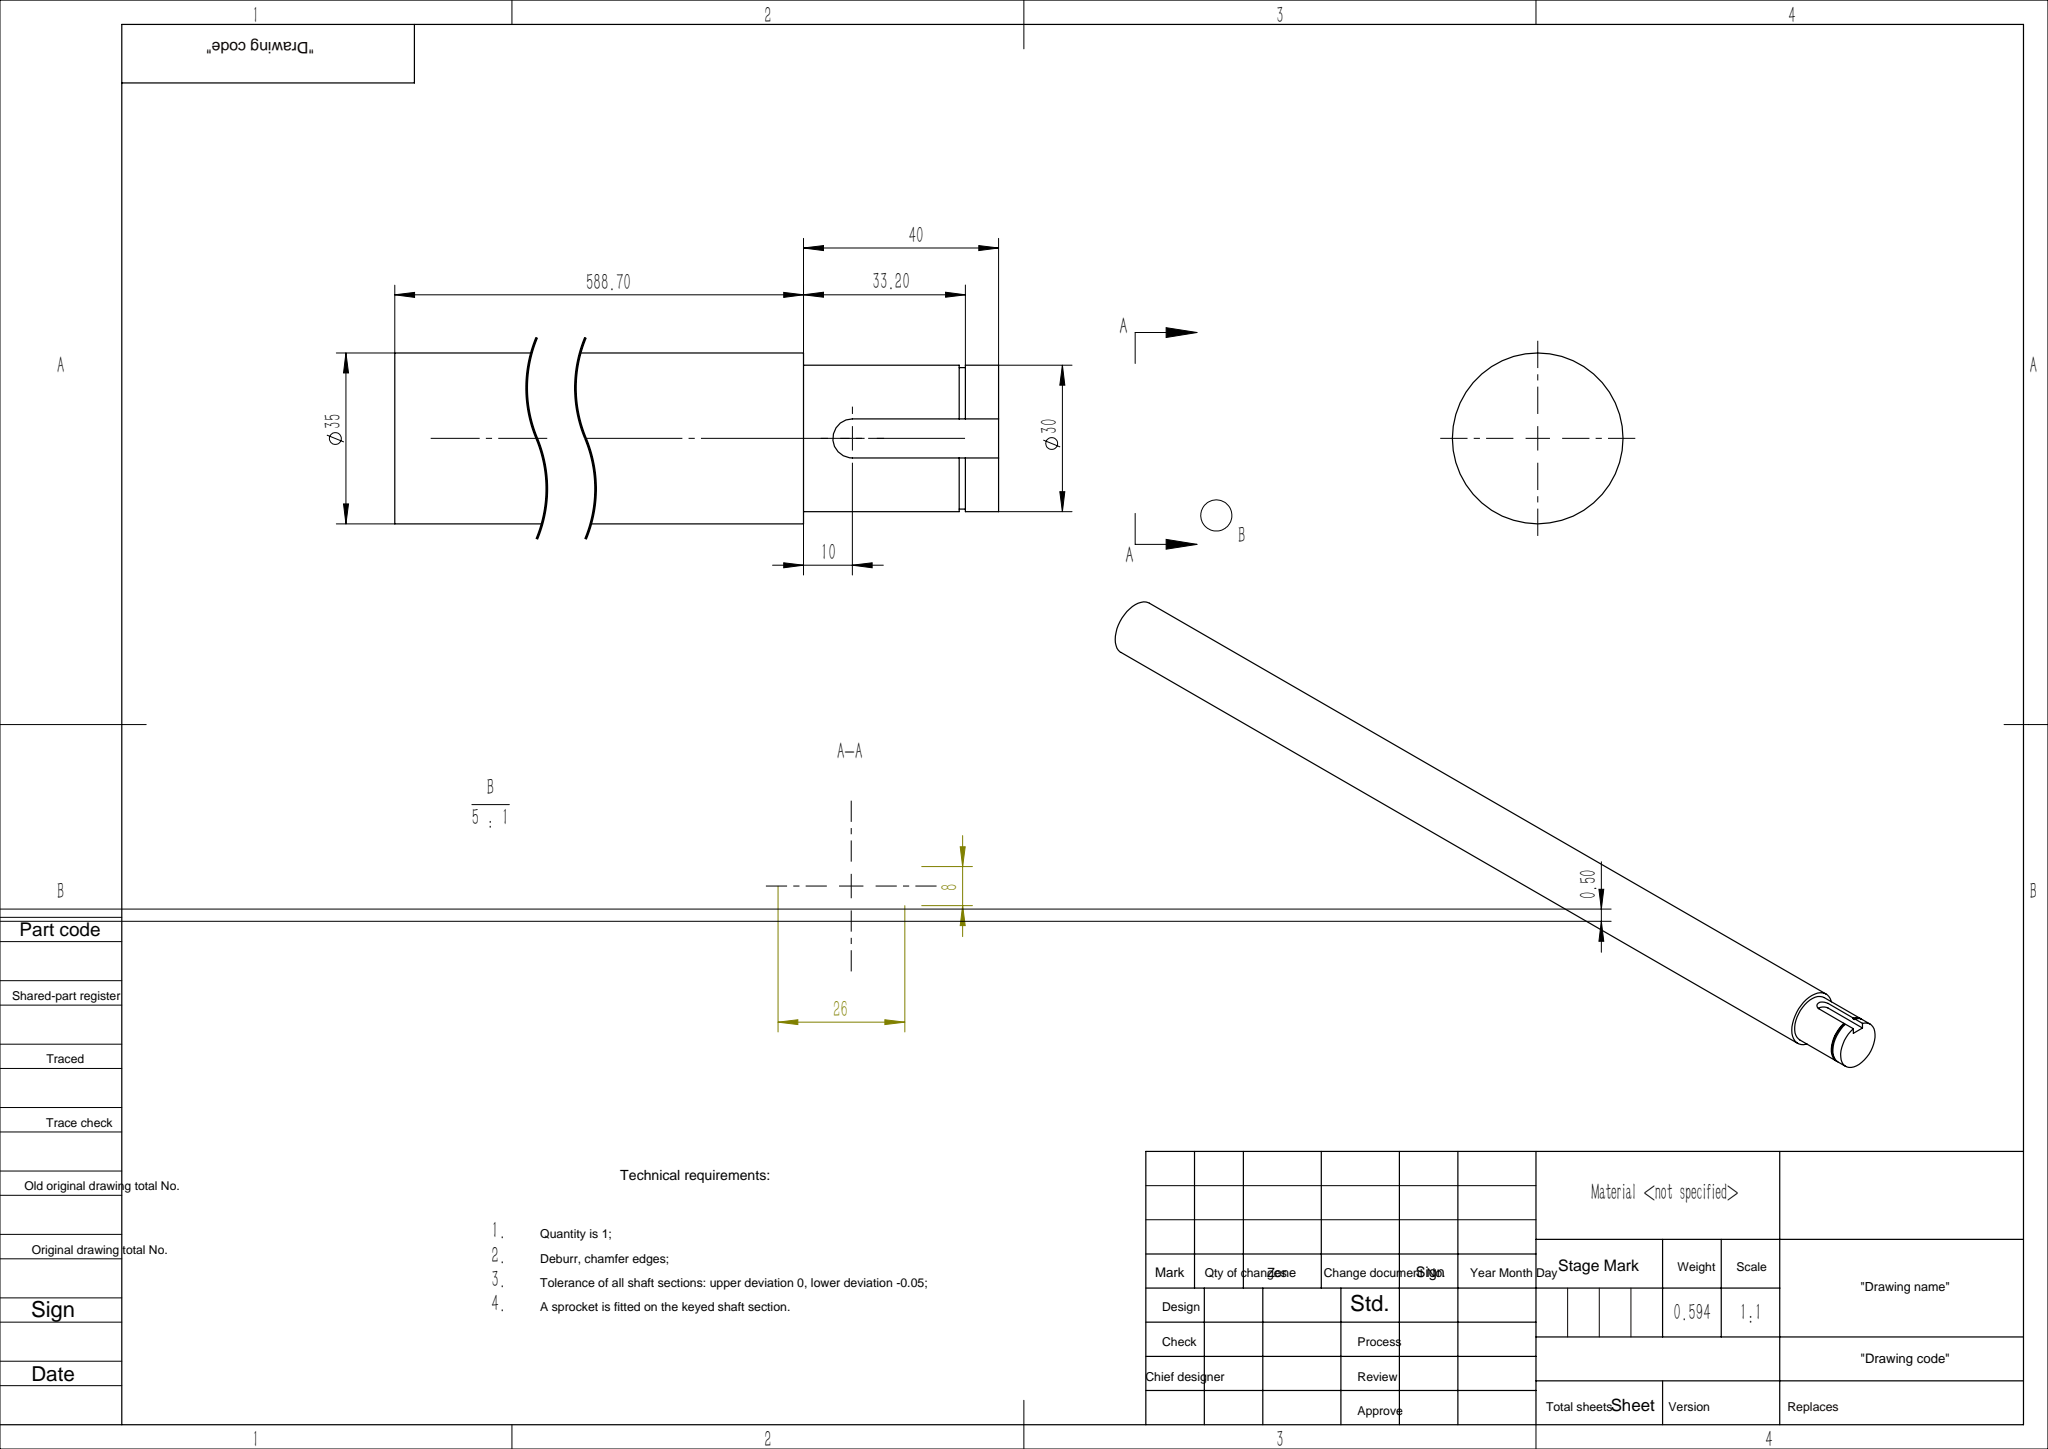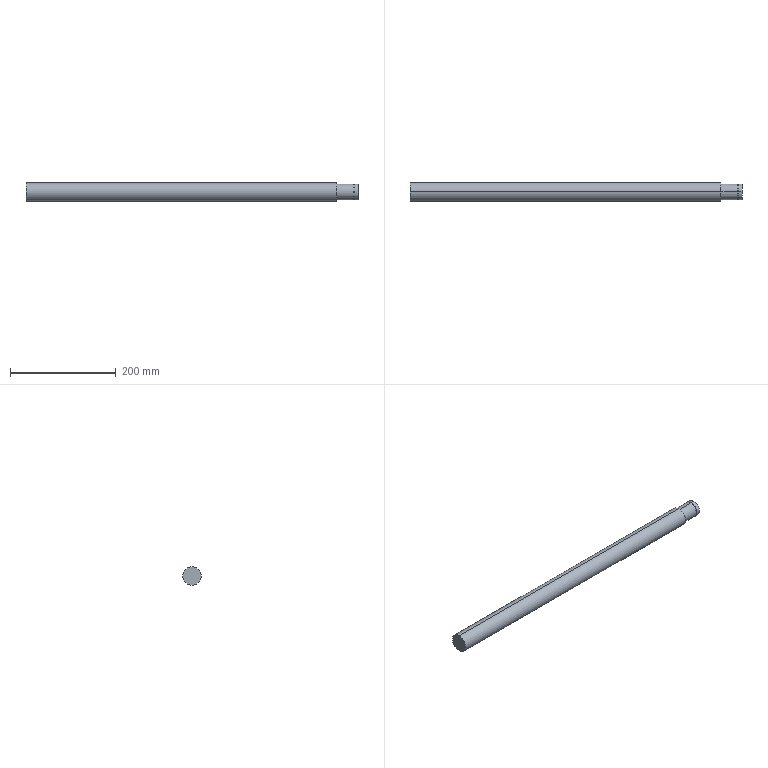Part | SolidWorks | features ICE 2, Cut 1, Extrusion 1 | 1 solid | 19 faces | box 628.7 x 35 x 35 mm | volume 593601 mm3 | cylinder 11 | plane 8 | commonest cylinder face diameters 30 x5 29 x3 35 x2 8 x1
STEP:
#1=CARTESIAN_POINT('',(620.6,13.937,4.));
#2=VERTEX_POINT('',#1);
#3=CARTESIAN_POINT('',(620.6,0.,14.5));
#4=VERTEX_POINT('',#3);
#5=CARTESIAN_POINT('',(620.6,0.,0.));
#6=DIRECTION('',(1.,0.,0.));
#7=DIRECTION('',(0.,0.,-1.));
#8=AXIS2_PLACEMENT_3D('',#5,#6,#7);
#9=CIRCLE('',#8,14.5);
#10=EDGE_CURVE('',#2,#4,#9,.T.);
#11=ORIENTED_EDGE('',*,*,#10,.T.);
#12=CARTESIAN_POINT('',(621.9,0.,14.5));
#13=VERTEX_POINT('',#12);
#14=CARTESIAN_POINT('',(620.6,0.,14.5));
#15=DIRECTION('',(1.,0.,0.));
#16=VECTOR('',#15,1000.);
#17=LINE('',#14,#16);
#18=EDGE_CURVE('',#4,#13,#17,.T.);
#19=ORIENTED_EDGE('',*,*,#18,.T.);
#20=CARTESIAN_POINT('',(621.9,13.937,4.));
#21=VERTEX_POINT('',#20);
#22=CARTESIAN_POINT('',(621.9,0.,0.));
#23=DIRECTION('',(1.,0.,0.));
#24=DIRECTION('',(0.,0.,-1.));
#25=AXIS2_PLACEMENT_3D('',#22,#23,#24);
#26=CIRCLE('',#25,14.5);
#27=EDGE_CURVE('',#21,#13,#26,.T.);
#28=ORIENTED_EDGE('',*,*,#27,.F.);
#29=CARTESIAN_POINT('',(620.6,13.937,4.));
#30=DIRECTION('',(-1.,0.,0.));
#31=VECTOR('',#30,1000.);
#32=LINE('',#29,#31);
#33=EDGE_CURVE('',#21,#2,#32,.T.);
#34=ORIENTED_EDGE('',*,*,#33,.T.);
#35=EDGE_LOOP('',(#11,#19,#28,#34));
#36=FACE_OUTER_BOUND('',#35,.T.);
#37=CARTESIAN_POINT('',(620.6,0.,0.));
#38=DIRECTION('',(1.,0.,0.));
#39=DIRECTION('',(0.,0.,-1.));
#40=AXIS2_PLACEMENT_3D('',#37,#38,#39);
#41=CYLINDRICAL_SURFACE('',#40,14.5);
#42=ADVANCED_FACE('',(#36),#41,.T.);
#43=ORIENTED_EDGE('',*,*,#18,.F.);
#44=CARTESIAN_POINT('',(620.6,0.,-14.5));
#45=VERTEX_POINT('',#44);
#46=CARTESIAN_POINT('',(620.6,0.,0.));
#47=DIRECTION('',(1.,0.,0.));
#48=DIRECTION('',(0.,0.,-1.));
#49=AXIS2_PLACEMENT_3D('',#46,#47,#48);
#50=CIRCLE('',#49,14.5);
#51=EDGE_CURVE('',#4,#45,#50,.T.);
#52=ORIENTED_EDGE('',*,*,#51,.T.);
#53=CARTESIAN_POINT('',(621.9,0.,-14.5));
#54=VERTEX_POINT('',#53);
#55=CARTESIAN_POINT('',(620.6,0.,-14.5));
#56=DIRECTION('',(1.,0.,0.));
#57=VECTOR('',#56,1000.);
#58=LINE('',#55,#57);
#59=EDGE_CURVE('',#45,#54,#58,.T.);
#60=ORIENTED_EDGE('',*,*,#59,.T.);
#61=CARTESIAN_POINT('',(621.9,0.,0.));
#62=DIRECTION('',(1.,0.,0.));
#63=DIRECTION('',(0.,0.,-1.));
#64=AXIS2_PLACEMENT_3D('',#61,#62,#63);
#65=CIRCLE('',#64,14.5);
#66=EDGE_CURVE('',#13,#54,#65,.T.);
#67=ORIENTED_EDGE('',*,*,#66,.F.);
#68=EDGE_LOOP('',(#43,#52,#60,#67));
#69=FACE_OUTER_BOUND('',#68,.T.);
#70=CARTESIAN_POINT('',(620.6,0.,0.));
#71=DIRECTION('',(1.,0.,0.));
#72=DIRECTION('',(0.,0.,-1.));
#73=AXIS2_PLACEMENT_3D('',#70,#71,#72);
#74=CYLINDRICAL_SURFACE('',#73,14.5);
#75=ADVANCED_FACE('',(#69),#74,.T.);
#76=CARTESIAN_POINT('',(621.9,14.457,4.));
#77=VERTEX_POINT('',#76);
#78=CARTESIAN_POINT('',(621.9,0.,15.));
#79=VERTEX_POINT('',#78);
#80=CARTESIAN_POINT('',(621.9,0.,0.));
#81=DIRECTION('',(1.,0.,0.));
#82=DIRECTION('',(0.,0.,-1.));
#83=AXIS2_PLACEMENT_3D('',#80,#81,#82);
#84=CIRCLE('',#83,15.);
#85=EDGE_CURVE('',#77,#79,#84,.T.);
#86=ORIENTED_EDGE('',*,*,#85,.T.);
#87=CARTESIAN_POINT('',(628.7,0.,15.));
#88=VERTEX_POINT('',#87);
#89=CARTESIAN_POINT('',(588.7,0.,15.));
#90=DIRECTION('',(1.,0.,0.));
#91=VECTOR('',#90,1000.);
#92=LINE('',#89,#91);
#93=EDGE_CURVE('',#79,#88,#92,.T.);
#94=ORIENTED_EDGE('',*,*,#93,.T.);
#95=CARTESIAN_POINT('',(628.7,14.457,4.));
#96=VERTEX_POINT('',#95);
#97=CARTESIAN_POINT('',(628.7,0.,0.));
#98=DIRECTION('',(1.,0.,0.));
#99=DIRECTION('',(0.,0.,-1.));
#100=AXIS2_PLACEMENT_3D('',#97,#98,#99);
#101=CIRCLE('',#100,15.);
#102=EDGE_CURVE('',#96,#88,#101,.T.);
#103=ORIENTED_EDGE('',*,*,#102,.F.);
#104=CARTESIAN_POINT('',(588.7,14.457,4.));
#105=DIRECTION('',(1.,0.,0.));
#106=VECTOR('',#105,1000.);
#107=LINE('',#104,#106);
#108=EDGE_CURVE('',#77,#96,#107,.T.);
#109=ORIENTED_EDGE('',*,*,#108,.F.);
#110=EDGE_LOOP('',(#86,#94,#103,#109));
#111=FACE_OUTER_BOUND('',#110,.T.);
#112=CARTESIAN_POINT('',(588.7,0.,0.));
#113=DIRECTION('',(1.,0.,0.));
#114=DIRECTION('',(0.,0.,-1.));
#115=AXIS2_PLACEMENT_3D('',#112,#113,#114);
#116=CYLINDRICAL_SURFACE('',#115,15.);
#117=ADVANCED_FACE('',(#111),#116,.T.);
#118=ORIENTED_EDGE('',*,*,#93,.F.);
#119=CARTESIAN_POINT('',(621.9,0.,-15.));
#120=VERTEX_POINT('',#119);
#121=CARTESIAN_POINT('',(621.9,0.,0.));
#122=DIRECTION('',(1.,0.,0.));
#123=DIRECTION('',(0.,0.,-1.));
#124=AXIS2_PLACEMENT_3D('',#121,#122,#123);
#125=CIRCLE('',#124,15.);
#126=EDGE_CURVE('',#79,#120,#125,.T.);
#127=ORIENTED_EDGE('',*,*,#126,.T.);
#128=CARTESIAN_POINT('',(628.7,0.,-15.));
#129=VERTEX_POINT('',#128);
#130=CARTESIAN_POINT('',(588.7,0.,-15.));
#131=DIRECTION('',(1.,0.,0.));
#132=VECTOR('',#131,1000.);
#133=LINE('',#130,#132);
#134=EDGE_CURVE('',#120,#129,#133,.T.);
#135=ORIENTED_EDGE('',*,*,#134,.T.);
#136=CARTESIAN_POINT('',(628.7,0.,0.));
#137=DIRECTION('',(1.,0.,0.));
#138=DIRECTION('',(0.,0.,-1.));
#139=AXIS2_PLACEMENT_3D('',#136,#137,#138);
#140=CIRCLE('',#139,15.);
#141=EDGE_CURVE('',#88,#129,#140,.T.);
#142=ORIENTED_EDGE('',*,*,#141,.F.);
#143=EDGE_LOOP('',(#118,#127,#135,#142));
#144=FACE_OUTER_BOUND('',#143,.T.);
#145=CARTESIAN_POINT('',(588.7,0.,0.));
#146=DIRECTION('',(1.,0.,0.));
#147=DIRECTION('',(0.,0.,-1.));
#148=AXIS2_PLACEMENT_3D('',#145,#146,#147);
#149=CYLINDRICAL_SURFACE('',#148,15.);
#150=ADVANCED_FACE('',(#144),#149,.T.);
#151=CARTESIAN_POINT('',(588.7,0.,-17.5));
#152=VERTEX_POINT('',#151);
#153=CARTESIAN_POINT('',(588.7,0.,17.5));
#154=VERTEX_POINT('',#153);
#155=CARTESIAN_POINT('',(588.7,0.,0.));
#156=DIRECTION('',(1.,0.,0.));
#157=DIRECTION('',(0.,0.,-1.));
#158=AXIS2_PLACEMENT_3D('',#155,#156,#157);
#159=CIRCLE('',#158,17.5);
#160=EDGE_CURVE('',#152,#154,#159,.T.);
#161=ORIENTED_EDGE('',*,*,#160,.F.);
#162=CARTESIAN_POINT('',(0.,0.,-17.5));
#163=VERTEX_POINT('',#162);
#164=CARTESIAN_POINT('',(628.7,0.,-17.5));
#165=DIRECTION('',(-1.,0.,0.));
#166=VECTOR('',#165,1000.);
#167=LINE('',#164,#166);
#168=EDGE_CURVE('',#152,#163,#167,.T.);
#169=ORIENTED_EDGE('',*,*,#168,.T.);
#170=CARTESIAN_POINT('',(0.,0.,17.5));
#171=VERTEX_POINT('',#170);
#172=CARTESIAN_POINT('',(0.,0.,0.));
#173=DIRECTION('',(1.,0.,0.));
#174=DIRECTION('',(0.,0.,-1.));
#175=AXIS2_PLACEMENT_3D('',#172,#173,#174);
#176=CIRCLE('',#175,17.5);
#177=EDGE_CURVE('',#163,#171,#176,.T.);
#178=ORIENTED_EDGE('',*,*,#177,.T.);
#179=CARTESIAN_POINT('',(628.7,0.,17.5));
#180=DIRECTION('',(-1.,0.,0.));
#181=VECTOR('',#180,1000.);
#182=LINE('',#179,#181);
#183=EDGE_CURVE('',#154,#171,#182,.T.);
#184=ORIENTED_EDGE('',*,*,#183,.F.);
#185=EDGE_LOOP('',(#161,#169,#178,#184));
#186=FACE_OUTER_BOUND('',#185,.T.);
#187=CARTESIAN_POINT('',(628.7,0.,0.));
#188=DIRECTION('',(-1.,0.,0.));
#189=DIRECTION('',(0.,0.,1.));
#190=AXIS2_PLACEMENT_3D('',#187,#188,#189);
#191=CYLINDRICAL_SURFACE('',#190,17.5);
#192=ADVANCED_FACE('',(#186),#191,.T.);
#193=CARTESIAN_POINT('',(588.7,0.,-15.));
#194=VERTEX_POINT('',#193);
#195=CARTESIAN_POINT('',(588.7,0.,15.));
#196=VERTEX_POINT('',#195);
#197=CARTESIAN_POINT('',(588.7,0.,0.));
#198=DIRECTION('',(1.,0.,0.));
#199=DIRECTION('',(0.,0.,-1.));
#200=AXIS2_PLACEMENT_3D('',#197,#198,#199);
#201=CIRCLE('',#200,15.);
#202=EDGE_CURVE('',#194,#196,#201,.T.);
#203=ORIENTED_EDGE('',*,*,#202,.T.);
#204=CARTESIAN_POINT('',(620.6,0.,15.));
#205=VERTEX_POINT('',#204);
#206=CARTESIAN_POINT('',(588.7,0.,15.));
#207=DIRECTION('',(1.,0.,0.));
#208=VECTOR('',#207,1000.);
#209=LINE('',#206,#208);
#210=EDGE_CURVE('',#196,#205,#209,.T.);
#211=ORIENTED_EDGE('',*,*,#210,.T.);
#212=CARTESIAN_POINT('',(620.6,14.457,4.));
#213=VERTEX_POINT('',#212);
#214=CARTESIAN_POINT('',(620.6,0.,0.));
#215=DIRECTION('',(1.,0.,0.));
#216=DIRECTION('',(0.,0.,-1.));
#217=AXIS2_PLACEMENT_3D('',#214,#215,#216);
#218=CIRCLE('',#217,15.);
#219=EDGE_CURVE('',#213,#205,#218,.T.);
#220=ORIENTED_EDGE('',*,*,#219,.F.);
#221=CARTESIAN_POINT('',(598.7,14.457,4.));
#222=VERTEX_POINT('',#221);
#223=CARTESIAN_POINT('',(588.7,14.457,4.));
#224=DIRECTION('',(1.,0.,0.));
#225=VECTOR('',#224,1000.);
#226=LINE('',#223,#225);
#227=EDGE_CURVE('',#222,#213,#226,.T.);
#228=ORIENTED_EDGE('',*,*,#227,.F.);
#229=CARTESIAN_POINT('',(598.7,14.457,-4.));
#230=VERTEX_POINT('',#229);
#231=CARTESIAN_POINT('',(598.7,14.457,-4.));
#232=CARTESIAN_POINT('',(598.434,14.457,-4.));
#233=CARTESIAN_POINT('',(598.174,14.464,-3.974));
#234=CARTESIAN_POINT('',(597.661,14.492,-3.872));
#235=CARTESIAN_POINT('',(597.406,14.513,-3.794));
#236=CARTESIAN_POINT('',(596.923,14.564,-3.593));
#237=CARTESIAN_POINT('',(596.693,14.594,-3.47));
#238=CARTESIAN_POINT('',(596.26,14.66,-3.18));
#239=CARTESIAN_POINT('',(596.055,14.696,-3.012));
#240=CARTESIAN_POINT('',(595.688,14.766,-2.645));
#241=CARTESIAN_POINT('',(595.523,14.801,-2.444));
#242=CARTESIAN_POINT('',(595.23,14.867,-2.008));
#243=CARTESIAN_POINT('',(595.107,14.896,-1.777));
#244=CARTESIAN_POINT('',(594.907,14.946,-1.296));
#245=CARTESIAN_POINT('',(594.829,14.966,-1.043));
#246=CARTESIAN_POINT('',(594.726,14.993,-0.5261));
#247=CARTESIAN_POINT('',(594.7,15.,-0.2658));
#248=CARTESIAN_POINT('',(594.7,15.,0.2585));
#249=CARTESIAN_POINT('',(594.726,14.993,0.5249));
#250=CARTESIAN_POINT('',(594.828,14.966,1.039));
#251=CARTESIAN_POINT('',(594.904,14.947,1.289));
#252=CARTESIAN_POINT('',(595.206,14.872,2.017));
#253=CARTESIAN_POINT('',(595.501,14.802,2.457));
#254=CARTESIAN_POINT('',(596.055,14.696,3.012));
#255=CARTESIAN_POINT('',(596.256,14.66,3.177));
#256=CARTESIAN_POINT('',(596.688,14.595,3.467));
#257=CARTESIAN_POINT('',(596.922,14.564,3.593));
#258=CARTESIAN_POINT('',(597.404,14.513,3.793));
#259=CARTESIAN_POINT('',(597.654,14.492,3.87));
#260=CARTESIAN_POINT('',(598.169,14.464,3.973));
#261=CARTESIAN_POINT('',(598.434,14.457,4.));
#262=CARTESIAN_POINT('',(598.7,14.457,4.));
#263=B_SPLINE_CURVE_WITH_KNOTS('',3,(#231,#232,#233,#234,#235,#236,#237,#238,#239,#240,#241,#242,#243,#244,#245,#246,#247,#248,#249,#250,#251,#252,#253,#254,#255,#256,#257,#258,#259,#260,#261,#262),.UNSPECIFIED.,.F.,.F.,(4,2,2,2,2,2,2,2,2,2,2,2,2,2,2,4),(0.,0.0007849,0.00157,0.002355,0.00314,0.003925,0.00471,0.005494,0.006279,0.007064,0.007849,0.009419,0.0102,0.01099,0.01177,0.01256),.UNSPECIFIED.);
#264=EDGE_CURVE('',#230,#222,#263,.T.);
#265=ORIENTED_EDGE('',*,*,#264,.F.);
#266=CARTESIAN_POINT('',(620.6,14.457,-4.));
#267=VERTEX_POINT('',#266);
#268=CARTESIAN_POINT('',(588.7,14.457,-4.));
#269=DIRECTION('',(-1.,0.,0.));
#270=VECTOR('',#269,1000.);
#271=LINE('',#268,#270);
#272=EDGE_CURVE('',#267,#230,#271,.T.);
#273=ORIENTED_EDGE('',*,*,#272,.F.);
#274=CARTESIAN_POINT('',(620.6,0.,-15.));
#275=VERTEX_POINT('',#274);
#276=CARTESIAN_POINT('',(620.6,0.,0.));
#277=DIRECTION('',(1.,0.,0.));
#278=DIRECTION('',(0.,0.,-1.));
#279=AXIS2_PLACEMENT_3D('',#276,#277,#278);
#280=CIRCLE('',#279,15.);
#281=EDGE_CURVE('',#275,#267,#280,.T.);
#282=ORIENTED_EDGE('',*,*,#281,.F.);
#283=CARTESIAN_POINT('',(588.7,0.,-15.));
#284=DIRECTION('',(1.,0.,0.));
#285=VECTOR('',#284,1000.);
#286=LINE('',#283,#285);
#287=EDGE_CURVE('',#194,#275,#286,.T.);
#288=ORIENTED_EDGE('',*,*,#287,.F.);
#289=EDGE_LOOP('',(#203,#211,#220,#228,#265,#273,#282,#288));
#290=FACE_OUTER_BOUND('',#289,.T.);
#291=CARTESIAN_POINT('',(588.7,0.,0.));
#292=DIRECTION('',(1.,0.,0.));
#293=DIRECTION('',(0.,0.,-1.));
#294=AXIS2_PLACEMENT_3D('',#291,#292,#293);
#295=CYLINDRICAL_SURFACE('',#294,15.);
#296=ADVANCED_FACE('',(#290),#295,.T.);
#297=ORIENTED_EDGE('',*,*,#210,.F.);
#298=CARTESIAN_POINT('',(588.7,0.,0.));
#299=DIRECTION('',(1.,0.,0.));
#300=DIRECTION('',(0.,0.,-1.));
#301=AXIS2_PLACEMENT_3D('',#298,#299,#300);
#302=CIRCLE('',#301,15.);
#303=EDGE_CURVE('',#196,#194,#302,.T.);
#304=ORIENTED_EDGE('',*,*,#303,.T.);
#305=ORIENTED_EDGE('',*,*,#287,.T.);
#306=CARTESIAN_POINT('',(620.6,0.,0.));
#307=DIRECTION('',(1.,0.,0.));
#308=DIRECTION('',(0.,0.,-1.));
#309=AXIS2_PLACEMENT_3D('',#306,#307,#308);
#310=CIRCLE('',#309,15.);
#311=EDGE_CURVE('',#205,#275,#310,.T.);
#312=ORIENTED_EDGE('',*,*,#311,.F.);
#313=EDGE_LOOP('',(#297,#304,#305,#312));
#314=FACE_OUTER_BOUND('',#313,.T.);
#315=CARTESIAN_POINT('',(588.7,0.,0.));
#316=DIRECTION('',(1.,0.,0.));
#317=DIRECTION('',(0.,0.,-1.));
#318=AXIS2_PLACEMENT_3D('',#315,#316,#317);
#319=CYLINDRICAL_SURFACE('',#318,15.);
#320=ADVANCED_FACE('',(#314),#319,.T.);
#321=CARTESIAN_POINT('',(620.6,13.937,-4.));
#322=VERTEX_POINT('',#321);
#323=CARTESIAN_POINT('',(620.6,11.,-4.));
#324=DIRECTION('',(0.,-1.,0.));
#325=VECTOR('',#324,1000.);
#326=LINE('',#323,#325);
#327=EDGE_CURVE('',#267,#322,#326,.T.);
#328=ORIENTED_EDGE('',*,*,#327,.F.);
#329=ORIENTED_EDGE('',*,*,#272,.T.);
#330=CARTESIAN_POINT('',(598.7,11.,-4.));
#331=VERTEX_POINT('',#330);
#332=CARTESIAN_POINT('',(598.7,11.,-4.));
#333=DIRECTION('',(0.,1.,0.));
#334=VECTOR('',#333,1000.);
#335=LINE('',#332,#334);
#336=EDGE_CURVE('',#331,#230,#335,.T.);
#337=ORIENTED_EDGE('',*,*,#336,.F.);
#338=CARTESIAN_POINT('',(628.7,11.,-4.));
#339=VERTEX_POINT('',#338);
#340=CARTESIAN_POINT('',(598.7,11.,-4.));
#341=DIRECTION('',(-1.,0.,0.));
#342=VECTOR('',#341,1000.);
#343=LINE('',#340,#342);
#344=EDGE_CURVE('',#339,#331,#343,.T.);
#345=ORIENTED_EDGE('',*,*,#344,.F.);
#346=CARTESIAN_POINT('',(628.7,14.457,-4.));
#347=VERTEX_POINT('',#346);
#348=CARTESIAN_POINT('',(628.7,11.,-4.));
#349=DIRECTION('',(0.,1.,0.));
#350=VECTOR('',#349,1000.);
#351=LINE('',#348,#350);
#352=EDGE_CURVE('',#339,#347,#351,.T.);
#353=ORIENTED_EDGE('',*,*,#352,.T.);
#354=CARTESIAN_POINT('',(621.9,14.457,-4.));
#355=VERTEX_POINT('',#354);
#356=CARTESIAN_POINT('',(588.7,14.457,-4.));
#357=DIRECTION('',(-1.,0.,0.));
#358=VECTOR('',#357,1000.);
#359=LINE('',#356,#358);
#360=EDGE_CURVE('',#347,#355,#359,.T.);
#361=ORIENTED_EDGE('',*,*,#360,.T.);
#362=CARTESIAN_POINT('',(621.9,13.937,-4.));
#363=VERTEX_POINT('',#362);
#364=CARTESIAN_POINT('',(621.9,11.,-4.));
#365=DIRECTION('',(0.,-1.,0.));
#366=VECTOR('',#365,1000.);
#367=LINE('',#364,#366);
#368=EDGE_CURVE('',#355,#363,#367,.T.);
#369=ORIENTED_EDGE('',*,*,#368,.T.);
#370=CARTESIAN_POINT('',(620.6,13.937,-4.));
#371=DIRECTION('',(1.,0.,0.));
#372=VECTOR('',#371,1000.);
#373=LINE('',#370,#372);
#374=EDGE_CURVE('',#322,#363,#373,.T.);
#375=ORIENTED_EDGE('',*,*,#374,.F.);
#376=EDGE_LOOP('',(#328,#329,#337,#345,#353,#361,#369,#375));
#377=FACE_OUTER_BOUND('',#376,.T.);
#378=CARTESIAN_POINT('',(598.7,11.,-4.));
#379=DIRECTION('',(0.,0.,-1.));
#380=DIRECTION('',(-1.,0.,0.));
#381=AXIS2_PLACEMENT_3D('',#378,#379,#380);
#382=PLANE('',#381);
#383=ADVANCED_FACE('',(#377),#382,.F.);
#384=CARTESIAN_POINT('',(620.6,11.,4.));
#385=DIRECTION('',(0.,1.,0.));
#386=VECTOR('',#385,1000.);
#387=LINE('',#384,#386);
#388=EDGE_CURVE('',#2,#213,#387,.T.);
#389=ORIENTED_EDGE('',*,*,#388,.F.);
#390=ORIENTED_EDGE('',*,*,#33,.F.);
#391=CARTESIAN_POINT('',(621.9,11.,4.));
#392=DIRECTION('',(0.,1.,0.));
#393=VECTOR('',#392,1000.);
#394=LINE('',#391,#393);
#395=EDGE_CURVE('',#21,#77,#394,.T.);
#396=ORIENTED_EDGE('',*,*,#395,.T.);
#397=ORIENTED_EDGE('',*,*,#108,.T.);
#398=CARTESIAN_POINT('',(628.7,11.,4.));
#399=VERTEX_POINT('',#398);
#400=CARTESIAN_POINT('',(628.7,11.,4.));
#401=DIRECTION('',(0.,1.,0.));
#402=VECTOR('',#401,1000.);
#403=LINE('',#400,#402);
#404=EDGE_CURVE('',#399,#96,#403,.T.);
#405=ORIENTED_EDGE('',*,*,#404,.F.);
#406=CARTESIAN_POINT('',(598.7,11.,4.));
#407=VERTEX_POINT('',#406);
#408=CARTESIAN_POINT('',(598.7,11.,4.));
#409=DIRECTION('',(1.,0.,0.));
#410=VECTOR('',#409,1000.);
#411=LINE('',#408,#410);
#412=EDGE_CURVE('',#407,#399,#411,.T.);
#413=ORIENTED_EDGE('',*,*,#412,.F.);
#414=CARTESIAN_POINT('',(598.7,11.,4.));
#415=DIRECTION('',(0.,1.,0.));
#416=VECTOR('',#415,1000.);
#417=LINE('',#414,#416);
#418=EDGE_CURVE('',#407,#222,#417,.T.);
#419=ORIENTED_EDGE('',*,*,#418,.T.);
#420=ORIENTED_EDGE('',*,*,#227,.T.);
#421=EDGE_LOOP('',(#389,#390,#396,#397,#405,#413,#419,#420));
#422=FACE_OUTER_BOUND('',#421,.T.);
#423=CARTESIAN_POINT('',(598.7,11.,4.));
#424=DIRECTION('',(0.,0.,1.));
#425=DIRECTION('',(1.,0.,0.));
#426=AXIS2_PLACEMENT_3D('',#423,#424,#425);
#427=PLANE('',#426);
#428=ADVANCED_FACE('',(#422),#427,.F.);
#429=ORIENTED_EDGE('',*,*,#168,.F.);
#430=CARTESIAN_POINT('',(588.7,0.,0.));
#431=DIRECTION('',(1.,0.,0.));
#432=DIRECTION('',(0.,0.,-1.));
#433=AXIS2_PLACEMENT_3D('',#430,#431,#432);
#434=CIRCLE('',#433,17.5);
#435=EDGE_CURVE('',#154,#152,#434,.T.);
#436=ORIENTED_EDGE('',*,*,#435,.F.);
#437=ORIENTED_EDGE('',*,*,#183,.T.);
#438=CARTESIAN_POINT('',(0.,0.,0.));
#439=DIRECTION('',(1.,0.,0.));
#440=DIRECTION('',(0.,0.,-1.));
#441=AXIS2_PLACEMENT_3D('',#438,#439,#440);
#442=CIRCLE('',#441,17.5);
#443=EDGE_CURVE('',#171,#163,#442,.T.);
#444=ORIENTED_EDGE('',*,*,#443,.T.);
#445=EDGE_LOOP('',(#429,#436,#437,#444));
#446=FACE_OUTER_BOUND('',#445,.T.);
#447=CARTESIAN_POINT('',(628.7,0.,0.));
#448=DIRECTION('',(-1.,0.,0.));
#449=DIRECTION('',(0.,0.,1.));
#450=AXIS2_PLACEMENT_3D('',#447,#448,#449);
#451=CYLINDRICAL_SURFACE('',#450,17.5);
#452=ADVANCED_FACE('',(#446),#451,.T.);
#453=ORIENTED_EDGE('',*,*,#443,.F.);
#454=ORIENTED_EDGE('',*,*,#177,.F.);
#455=EDGE_LOOP('',(#453,#454));
#456=FACE_OUTER_BOUND('',#455,.T.);
#457=CARTESIAN_POINT('',(0.,0.,0.));
#458=DIRECTION('',(1.,0.,0.));
#459=DIRECTION('',(0.,0.,-1.));
#460=AXIS2_PLACEMENT_3D('',#457,#458,#459);
#461=PLANE('',#460);
#462=ADVANCED_FACE('',(#456),#461,.F.);
#463=ORIENTED_EDGE('',*,*,#202,.F.);
#464=ORIENTED_EDGE('',*,*,#303,.F.);
#465=EDGE_LOOP('',(#463,#464));
#466=FACE_BOUND('',#465,.T.);
#467=ORIENTED_EDGE('',*,*,#435,.T.);
#468=ORIENTED_EDGE('',*,*,#160,.T.);
#469=EDGE_LOOP('',(#467,#468));
#470=FACE_OUTER_BOUND('',#469,.T.);
#471=CARTESIAN_POINT('',(588.7,0.,0.));
#472=DIRECTION('',(1.,0.,0.));
#473=DIRECTION('',(0.,0.,-1.));
#474=AXIS2_PLACEMENT_3D('',#471,#472,#473);
#475=PLANE('',#474);
#476=ADVANCED_FACE('',(#466,#470),#475,.T.);
#477=ORIENTED_EDGE('',*,*,#134,.F.);
#478=CARTESIAN_POINT('',(621.9,0.,0.));
#479=DIRECTION('',(1.,0.,0.));
#480=DIRECTION('',(0.,0.,-1.));
#481=AXIS2_PLACEMENT_3D('',#478,#479,#480);
#482=CIRCLE('',#481,15.);
#483=EDGE_CURVE('',#120,#355,#482,.T.);
#484=ORIENTED_EDGE('',*,*,#483,.T.);
#485=ORIENTED_EDGE('',*,*,#360,.F.);
#486=CARTESIAN_POINT('',(628.7,0.,0.));
#487=DIRECTION('',(1.,0.,0.));
#488=DIRECTION('',(0.,0.,-1.));
#489=AXIS2_PLACEMENT_3D('',#486,#487,#488);
#490=CIRCLE('',#489,15.);
#491=EDGE_CURVE('',#129,#347,#490,.T.);
#492=ORIENTED_EDGE('',*,*,#491,.F.);
#493=EDGE_LOOP('',(#477,#484,#485,#492));
#494=FACE_OUTER_BOUND('',#493,.T.);
#495=CARTESIAN_POINT('',(588.7,0.,0.));
#496=DIRECTION('',(1.,0.,0.));
#497=DIRECTION('',(0.,0.,-1.));
#498=AXIS2_PLACEMENT_3D('',#495,#496,#497);
#499=CYLINDRICAL_SURFACE('',#498,15.);
#500=ADVANCED_FACE('',(#494),#499,.T.);
#501=ORIENTED_EDGE('',*,*,#352,.F.);
#502=CARTESIAN_POINT('',(628.7,11.,-4.));
#503=DIRECTION('',(0.,0.,-1.));
#504=VECTOR('',#503,1000.);
#505=LINE('',#502,#504);
#506=EDGE_CURVE('',#399,#339,#505,.T.);
#507=ORIENTED_EDGE('',*,*,#506,.F.);
#508=ORIENTED_EDGE('',*,*,#404,.T.);
#509=ORIENTED_EDGE('',*,*,#102,.T.);
#510=ORIENTED_EDGE('',*,*,#141,.T.);
#511=ORIENTED_EDGE('',*,*,#491,.T.);
#512=EDGE_LOOP('',(#501,#507,#508,#509,#510,#511));
#513=FACE_OUTER_BOUND('',#512,.T.);
#514=CARTESIAN_POINT('',(628.7,0.,0.));
#515=DIRECTION('',(1.,0.,0.));
#516=DIRECTION('',(0.,0.,-1.));
#517=AXIS2_PLACEMENT_3D('',#514,#515,#516);
#518=PLANE('',#517);
#519=ADVANCED_FACE('',(#513),#518,.T.);
#520=ORIENTED_EDGE('',*,*,#336,.T.);
#521=ORIENTED_EDGE('',*,*,#264,.T.);
#522=ORIENTED_EDGE('',*,*,#418,.F.);
#523=CARTESIAN_POINT('',(598.7,11.,0.));
#524=DIRECTION('',(0.,1.,0.));
#525=DIRECTION('',(0.,0.,1.));
#526=AXIS2_PLACEMENT_3D('',#523,#524,#525);
#527=CIRCLE('',#526,4.);
#528=EDGE_CURVE('',#331,#407,#527,.T.);
#529=ORIENTED_EDGE('',*,*,#528,.F.);
#530=EDGE_LOOP('',(#520,#521,#522,#529));
#531=FACE_OUTER_BOUND('',#530,.T.);
#532=CARTESIAN_POINT('',(598.7,11.,0.));
#533=DIRECTION('',(0.,1.,0.));
#534=DIRECTION('',(0.,0.,1.));
#535=AXIS2_PLACEMENT_3D('',#532,#533,#534);
#536=CYLINDRICAL_SURFACE('',#535,4.);
#537=ADVANCED_FACE('',(#531),#536,.F.);
#538=ORIENTED_EDGE('',*,*,#528,.T.);
#539=ORIENTED_EDGE('',*,*,#412,.T.);
#540=ORIENTED_EDGE('',*,*,#506,.T.);
#541=ORIENTED_EDGE('',*,*,#344,.T.);
#542=EDGE_LOOP('',(#538,#539,#540,#541));
#543=FACE_OUTER_BOUND('',#542,.T.);
#544=CARTESIAN_POINT('',(598.7,11.,0.));
#545=DIRECTION('',(0.,1.,0.));
#546=DIRECTION('',(0.,0.,1.));
#547=AXIS2_PLACEMENT_3D('',#544,#545,#546);
#548=PLANE('',#547);
#549=ADVANCED_FACE('',(#543),#548,.T.);
#550=ORIENTED_EDGE('',*,*,#327,.T.);
#551=CARTESIAN_POINT('',(620.6,0.,0.));
#552=DIRECTION('',(1.,0.,0.));
#553=DIRECTION('',(0.,0.,-1.));
#554=AXIS2_PLACEMENT_3D('',#551,#552,#553);
#555=CIRCLE('',#554,14.5);
#556=EDGE_CURVE('',#45,#322,#555,.T.);
#557=ORIENTED_EDGE('',*,*,#556,.F.);
#558=ORIENTED_EDGE('',*,*,#51,.F.);
#559=ORIENTED_EDGE('',*,*,#10,.F.);
#560=ORIENTED_EDGE('',*,*,#388,.T.);
#561=ORIENTED_EDGE('',*,*,#219,.T.);
#562=ORIENTED_EDGE('',*,*,#311,.T.);
#563=ORIENTED_EDGE('',*,*,#281,.T.);
#564=EDGE_LOOP('',(#550,#557,#558,#559,#560,#561,#562,#563));
#565=FACE_OUTER_BOUND('',#564,.T.);
#566=CARTESIAN_POINT('',(620.6,0.,0.));
#567=DIRECTION('',(1.,0.,0.));
#568=DIRECTION('',(0.,0.,-1.));
#569=AXIS2_PLACEMENT_3D('',#566,#567,#568);
#570=PLANE('',#569);
#571=ADVANCED_FACE('',(#565),#570,.T.);
#572=ORIENTED_EDGE('',*,*,#85,.F.);
#573=ORIENTED_EDGE('',*,*,#395,.F.);
#574=ORIENTED_EDGE('',*,*,#27,.T.);
#575=ORIENTED_EDGE('',*,*,#66,.T.);
#576=CARTESIAN_POINT('',(621.9,0.,0.));
#577=DIRECTION('',(1.,0.,0.));
#578=DIRECTION('',(0.,0.,-1.));
#579=AXIS2_PLACEMENT_3D('',#576,#577,#578);
#580=CIRCLE('',#579,14.5);
#581=EDGE_CURVE('',#54,#363,#580,.T.);
#582=ORIENTED_EDGE('',*,*,#581,.T.);
#583=ORIENTED_EDGE('',*,*,#368,.F.);
#584=ORIENTED_EDGE('',*,*,#483,.F.);
#585=ORIENTED_EDGE('',*,*,#126,.F.);
#586=EDGE_LOOP('',(#572,#573,#574,#575,#582,#583,#584,#585));
#587=FACE_OUTER_BOUND('',#586,.T.);
#588=CARTESIAN_POINT('',(621.9,0.,0.));
#589=DIRECTION('',(1.,0.,0.));
#590=DIRECTION('',(0.,0.,-1.));
#591=AXIS2_PLACEMENT_3D('',#588,#589,#590);
#592=PLANE('',#591);
#593=ADVANCED_FACE('',(#587),#592,.F.);
#594=ORIENTED_EDGE('',*,*,#59,.F.);
#595=ORIENTED_EDGE('',*,*,#556,.T.);
#596=ORIENTED_EDGE('',*,*,#374,.T.);
#597=ORIENTED_EDGE('',*,*,#581,.F.);
#598=EDGE_LOOP('',(#594,#595,#596,#597));
#599=FACE_OUTER_BOUND('',#598,.T.);
#600=CARTESIAN_POINT('',(620.6,0.,0.));
#601=DIRECTION('',(1.,0.,0.));
#602=DIRECTION('',(0.,0.,-1.));
#603=AXIS2_PLACEMENT_3D('',#600,#601,#602);
#604=CYLINDRICAL_SURFACE('',#603,14.5);
#605=ADVANCED_FACE('',(#599),#604,.T.);
#606=CLOSED_SHELL('',(#42,#75,#117,#150,#192,#296,#320,#383,#428,#452,#462,#476,#500,#519,#537,#549,#571,#593,#605));
#607=MANIFOLD_SOLID_BREP('',#606);
#608=CARTESIAN_POINT('',(0.,0.,0.));
#609=DIRECTION('',(0.,0.,1.));
#610=DIRECTION('',(1.,0.,0.));
#611=AXIS2_PLACEMENT_3D('',#608,#609,#610);
#612=(LENGTH_UNIT()NAMED_UNIT(*)SI_UNIT(.MILLI.,.METRE.));
#613=UNCERTAINTY_MEASURE_WITH_UNIT(LENGTH_MEASURE(0.00001),#612,'','');
#614=(NAMED_UNIT(*)PLANE_ANGLE_UNIT()SI_UNIT($,.RADIAN.));
#615=(NAMED_UNIT(*)SI_UNIT($,.STERADIAN.)SOLID_ANGLE_UNIT());
#616=(GEOMETRIC_REPRESENTATION_CONTEXT(3)GLOBAL_UNCERTAINTY_ASSIGNED_CONTEXT((#613))GLOBAL_UNIT_ASSIGNED_CONTEXT((#612,#614,#615))REPRESENTATION_CONTEXT('',''));
#617=ADVANCED_BREP_SHAPE_REPRESENTATION('',(#607,#611),#616);